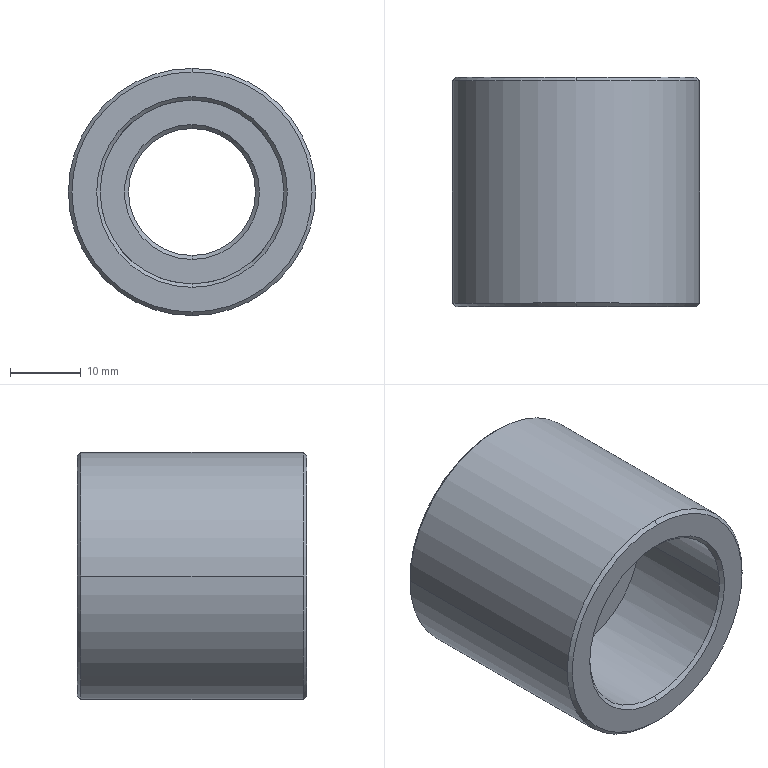Part | Creo | 1 solid | 17 faces | box 35 x 32.5 x 35 mm | volume 18391 mm3 | cone 8 | cylinder 6 | plane 3 | commonest cylinder face diameters 18 x2 26 x2 35 x2
STEP:
#1=CARTESIAN_POINT('',(203.5,-339.005,-225.));
#2=VERTEX_POINT('',#1);
#3=CARTESIAN_POINT('',(212.5,-339.005,-234.));
#4=VERTEX_POINT('',#3);
#5=CARTESIAN_POINT('',(212.5,-339.005,-225.));
#6=DIRECTION('',(0.,-1.,0.));
#7=DIRECTION('',(-1.,0.,0.));
#8=AXIS2_PLACEMENT_3D('',#5,#6,#7);
#9=CIRCLE('',#8,9.);
#10=EDGE_CURVE('',#2,#4,#9,.T.);
#11=ORIENTED_EDGE('',*,*,#10,.T.);
#12=CARTESIAN_POINT('',(221.5,-339.005,-225.));
#13=VERTEX_POINT('',#12);
#14=CARTESIAN_POINT('',(212.5,-339.005,-225.));
#15=DIRECTION('',(0.,-1.,0.));
#16=DIRECTION('',(0.,0.,-1.));
#17=AXIS2_PLACEMENT_3D('',#14,#15,#16);
#18=CIRCLE('',#17,9.);
#19=EDGE_CURVE('',#4,#13,#18,.T.);
#20=ORIENTED_EDGE('',*,*,#19,.T.);
#21=CARTESIAN_POINT('',(221.5,-354.455,-225.));
#22=VERTEX_POINT('',#21);
#23=CARTESIAN_POINT('',(221.5,-339.005,-225.));
#24=DIRECTION('',(0.,-1.,0.));
#25=VECTOR('',#24,15.45);
#26=LINE('',#23,#25);
#27=EDGE_CURVE('',#13,#22,#26,.T.);
#28=ORIENTED_EDGE('',*,*,#27,.T.);
#29=CARTESIAN_POINT('',(212.5,-354.455,-234.));
#30=VERTEX_POINT('',#29);
#31=CARTESIAN_POINT('',(212.5,-354.455,-225.));
#32=DIRECTION('',(0.,1.,0.));
#33=DIRECTION('',(1.,0.,0.));
#34=AXIS2_PLACEMENT_3D('',#31,#32,#33);
#35=CIRCLE('',#34,9.);
#36=EDGE_CURVE('',#22,#30,#35,.T.);
#37=ORIENTED_EDGE('',*,*,#36,.T.);
#38=CARTESIAN_POINT('',(203.5,-354.455,-225.));
#39=VERTEX_POINT('',#38);
#40=CARTESIAN_POINT('',(212.5,-354.455,-225.));
#41=DIRECTION('',(0.,1.,0.));
#42=DIRECTION('',(0.,0.,-1.));
#43=AXIS2_PLACEMENT_3D('',#40,#41,#42);
#44=CIRCLE('',#43,9.);
#45=EDGE_CURVE('',#30,#39,#44,.T.);
#46=ORIENTED_EDGE('',*,*,#45,.T.);
#47=CARTESIAN_POINT('',(203.5,-339.005,-225.));
#48=DIRECTION('',(0.,-1.,0.));
#49=VECTOR('',#48,15.45);
#50=LINE('',#47,#49);
#51=EDGE_CURVE('',#2,#39,#50,.T.);
#52=ORIENTED_EDGE('',*,*,#51,.F.);
#53=EDGE_LOOP('',(#11,#20,#28,#37,#46,#52));
#54=FACE_OUTER_BOUND('',#53,.F.);
#55=CARTESIAN_POINT('',(212.5,-374.005,-225.));
#56=DIRECTION('',(0.,-1.,0.));
#57=DIRECTION('',(-1.,0.,0.));
#58=AXIS2_PLACEMENT_3D('',#55,#56,#57);
#59=CYLINDRICAL_SURFACE('',#58,9.);
#60=ADVANCED_FACE('',(#54),#59,.F.);
#61=CARTESIAN_POINT('',(229.5,-339.005,-225.));
#62=VERTEX_POINT('',#61);
#63=CARTESIAN_POINT('',(212.5,-339.005,-242.));
#64=VERTEX_POINT('',#63);
#65=CARTESIAN_POINT('',(212.5,-339.005,-225.));
#66=DIRECTION('',(0.,1.,0.));
#67=DIRECTION('',(1.,0.,0.));
#68=AXIS2_PLACEMENT_3D('',#65,#66,#67);
#69=CIRCLE('',#68,17.);
#70=EDGE_CURVE('',#62,#64,#69,.T.);
#71=ORIENTED_EDGE('',*,*,#70,.F.);
#72=CARTESIAN_POINT('',(212.5,-339.005,-208.));
#73=VERTEX_POINT('',#72);
#74=CARTESIAN_POINT('',(212.5,-339.005,-225.));
#75=DIRECTION('',(0.,1.,0.));
#76=DIRECTION('',(0.,0.,1.));
#77=AXIS2_PLACEMENT_3D('',#74,#75,#76);
#78=CIRCLE('',#77,17.);
#79=EDGE_CURVE('',#73,#62,#78,.T.);
#80=ORIENTED_EDGE('',*,*,#79,.F.);
#81=CARTESIAN_POINT('',(195.5,-339.005,-225.));
#82=VERTEX_POINT('',#81);
#83=CARTESIAN_POINT('',(212.5,-339.005,-225.));
#84=DIRECTION('',(0.,1.,0.));
#85=DIRECTION('',(-1.,0.,0.));
#86=AXIS2_PLACEMENT_3D('',#83,#84,#85);
#87=CIRCLE('',#86,17.);
#88=EDGE_CURVE('',#82,#73,#87,.T.);
#89=ORIENTED_EDGE('',*,*,#88,.F.);
#90=CARTESIAN_POINT('',(212.5,-339.005,-225.));
#91=DIRECTION('',(0.,1.,0.));
#92=DIRECTION('',(0.,0.,-1.));
#93=AXIS2_PLACEMENT_3D('',#90,#91,#92);
#94=CIRCLE('',#93,17.);
#95=EDGE_CURVE('',#64,#82,#94,.T.);
#96=ORIENTED_EDGE('',*,*,#95,.F.);
#97=EDGE_LOOP('',(#71,#80,#89,#96));
#98=FACE_OUTER_BOUND('',#97,.F.);
#99=ORIENTED_EDGE('',*,*,#19,.F.);
#100=ORIENTED_EDGE('',*,*,#10,.F.);
#101=CARTESIAN_POINT('',(212.5,-339.005,-216.));
#102=VERTEX_POINT('',#101);
#103=CARTESIAN_POINT('',(212.5,-339.005,-225.));
#104=DIRECTION('',(0.,-1.,0.));
#105=DIRECTION('',(0.,0.,1.));
#106=AXIS2_PLACEMENT_3D('',#103,#104,#105);
#107=CIRCLE('',#106,9.);
#108=EDGE_CURVE('',#102,#2,#107,.T.);
#109=ORIENTED_EDGE('',*,*,#108,.F.);
#110=CARTESIAN_POINT('',(212.5,-339.005,-225.));
#111=DIRECTION('',(0.,-1.,0.));
#112=DIRECTION('',(1.,0.,0.));
#113=AXIS2_PLACEMENT_3D('',#110,#111,#112);
#114=CIRCLE('',#113,9.);
#115=EDGE_CURVE('',#13,#102,#114,.T.);
#116=ORIENTED_EDGE('',*,*,#115,.F.);
#117=EDGE_LOOP('',(#99,#100,#109,#116));
#118=FACE_BOUND('',#117,.F.);
#119=CARTESIAN_POINT('',(250.,-339.005,-375.));
#120=DIRECTION('',(0.,-1.,0.));
#121=DIRECTION('',(-1.,0.,0.));
#122=AXIS2_PLACEMENT_3D('',#119,#120,#121);
#123=PLANE('',#122);
#124=ADVANCED_FACE('',(#98,#118),#123,.F.);
#125=ORIENTED_EDGE('',*,*,#108,.T.);
#126=ORIENTED_EDGE('',*,*,#51,.T.);
#127=CARTESIAN_POINT('',(212.5,-354.455,-216.));
#128=VERTEX_POINT('',#127);
#129=CARTESIAN_POINT('',(212.5,-354.455,-225.));
#130=DIRECTION('',(0.,1.,0.));
#131=DIRECTION('',(-1.,0.,0.));
#132=AXIS2_PLACEMENT_3D('',#129,#130,#131);
#133=CIRCLE('',#132,9.);
#134=EDGE_CURVE('',#39,#128,#133,.T.);
#135=ORIENTED_EDGE('',*,*,#134,.T.);
#136=CARTESIAN_POINT('',(212.5,-354.455,-225.));
#137=DIRECTION('',(0.,1.,0.));
#138=DIRECTION('',(0.,0.,1.));
#139=AXIS2_PLACEMENT_3D('',#136,#137,#138);
#140=CIRCLE('',#139,9.);
#141=EDGE_CURVE('',#128,#22,#140,.T.);
#142=ORIENTED_EDGE('',*,*,#141,.T.);
#143=ORIENTED_EDGE('',*,*,#27,.F.);
#144=ORIENTED_EDGE('',*,*,#115,.T.);
#145=EDGE_LOOP('',(#125,#126,#135,#142,#143,#144));
#146=FACE_OUTER_BOUND('',#145,.F.);
#147=CARTESIAN_POINT('',(212.5,-374.005,-225.));
#148=DIRECTION('',(0.,-1.,0.));
#149=DIRECTION('',(-1.,0.,0.));
#150=AXIS2_PLACEMENT_3D('',#147,#148,#149);
#151=CYLINDRICAL_SURFACE('',#150,9.);
#152=ADVANCED_FACE('',(#146),#151,.F.);
#153=ORIENTED_EDGE('',*,*,#45,.F.);
#154=CARTESIAN_POINT('',(212.5,-355.005,-234.55));
#155=VERTEX_POINT('',#154);
#156=CARTESIAN_POINT('',(212.5,-354.455,-234.));
#157=DIRECTION('',(0.,-0.7071,-0.7071));
#158=VECTOR('',#157,0.7778);
#159=LINE('',#156,#158);
#160=EDGE_CURVE('',#30,#155,#159,.T.);
#161=ORIENTED_EDGE('',*,*,#160,.T.);
#162=CARTESIAN_POINT('',(212.5,-355.005,-215.45));
#163=VERTEX_POINT('',#162);
#164=CARTESIAN_POINT('',(212.5,-355.005,-225.));
#165=DIRECTION('',(0.,1.,0.));
#166=DIRECTION('',(0.,0.,-1.));
#167=AXIS2_PLACEMENT_3D('',#164,#165,#166);
#168=CIRCLE('',#167,9.55);
#169=EDGE_CURVE('',#155,#163,#168,.T.);
#170=ORIENTED_EDGE('',*,*,#169,.T.);
#171=CARTESIAN_POINT('',(212.5,-354.455,-216.));
#172=DIRECTION('',(0.,-0.7071,0.7071));
#173=VECTOR('',#172,0.7778);
#174=LINE('',#171,#173);
#175=EDGE_CURVE('',#128,#163,#174,.T.);
#176=ORIENTED_EDGE('',*,*,#175,.F.);
#177=ORIENTED_EDGE('',*,*,#134,.F.);
#178=EDGE_LOOP('',(#153,#161,#170,#176,#177));
#179=FACE_OUTER_BOUND('',#178,.F.);
#180=CARTESIAN_POINT('',(212.5,-354.73,-225.));
#181=DIRECTION('',(0.,-1.,0.));
#182=DIRECTION('',(0.,0.,1.));
#183=AXIS2_PLACEMENT_3D('',#180,#181,#182);
#184=CONICAL_SURFACE('',#183,9.275,45.);
#185=ADVANCED_FACE('',(#179),#184,.F.);
#186=ORIENTED_EDGE('',*,*,#141,.F.);
#187=ORIENTED_EDGE('',*,*,#175,.T.);
#188=CARTESIAN_POINT('',(222.05,-355.005,-225.));
#189=VERTEX_POINT('',#188);
#190=CARTESIAN_POINT('',(212.5,-355.005,-225.));
#191=DIRECTION('',(0.,1.,0.));
#192=DIRECTION('',(0.,0.,1.));
#193=AXIS2_PLACEMENT_3D('',#190,#191,#192);
#194=CIRCLE('',#193,9.55);
#195=EDGE_CURVE('',#163,#189,#194,.T.);
#196=ORIENTED_EDGE('',*,*,#195,.T.);
#197=CARTESIAN_POINT('',(212.5,-355.005,-225.));
#198=DIRECTION('',(0.,1.,0.));
#199=DIRECTION('',(1.,0.,0.));
#200=AXIS2_PLACEMENT_3D('',#197,#198,#199);
#201=CIRCLE('',#200,9.55);
#202=EDGE_CURVE('',#189,#155,#201,.T.);
#203=ORIENTED_EDGE('',*,*,#202,.T.);
#204=ORIENTED_EDGE('',*,*,#160,.F.);
#205=ORIENTED_EDGE('',*,*,#36,.F.);
#206=EDGE_LOOP('',(#186,#187,#196,#203,#204,#205));
#207=FACE_OUTER_BOUND('',#206,.F.);
#208=CARTESIAN_POINT('',(212.5,-354.73,-225.));
#209=DIRECTION('',(0.,-1.,0.));
#210=DIRECTION('',(0.,0.,1.));
#211=AXIS2_PLACEMENT_3D('',#208,#209,#210);
#212=CONICAL_SURFACE('',#211,9.275,45.);
#213=ADVANCED_FACE('',(#207),#212,.F.);
#214=CARTESIAN_POINT('',(199.5,-355.005,-225.));
#215=VERTEX_POINT('',#214);
#216=CARTESIAN_POINT('',(225.5,-355.005,-225.));
#217=VERTEX_POINT('',#216);
#218=CARTESIAN_POINT('',(212.5,-355.005,-225.));
#219=DIRECTION('',(0.,-1.,0.));
#220=DIRECTION('',(-1.,0.,0.));
#221=AXIS2_PLACEMENT_3D('',#218,#219,#220);
#222=CIRCLE('',#221,13.);
#223=EDGE_CURVE('',#215,#217,#222,.T.);
#224=ORIENTED_EDGE('',*,*,#223,.F.);
#225=CARTESIAN_POINT('',(212.5,-355.005,-225.));
#226=DIRECTION('',(0.,-1.,0.));
#227=DIRECTION('',(1.,0.,0.));
#228=AXIS2_PLACEMENT_3D('',#225,#226,#227);
#229=CIRCLE('',#228,13.);
#230=EDGE_CURVE('',#217,#215,#229,.T.);
#231=ORIENTED_EDGE('',*,*,#230,.F.);
#232=EDGE_LOOP('',(#224,#231));
#233=FACE_OUTER_BOUND('',#232,.F.);
#234=ORIENTED_EDGE('',*,*,#202,.F.);
#235=ORIENTED_EDGE('',*,*,#195,.F.);
#236=ORIENTED_EDGE('',*,*,#169,.F.);
#237=EDGE_LOOP('',(#234,#235,#236));
#238=FACE_BOUND('',#237,.F.);
#239=CARTESIAN_POINT('',(250.,-355.005,-375.));
#240=DIRECTION('',(0.,-1.,0.));
#241=DIRECTION('',(-1.,0.,0.));
#242=AXIS2_PLACEMENT_3D('',#239,#240,#241);
#243=PLANE('',#242);
#244=ADVANCED_FACE('',(#233,#238),#243,.T.);
#245=CARTESIAN_POINT('',(212.5,-371.005,-238.));
#246=VERTEX_POINT('',#245);
#247=CARTESIAN_POINT('',(199.5,-371.005,-225.));
#248=VERTEX_POINT('',#247);
#249=CARTESIAN_POINT('',(212.5,-371.005,-225.));
#250=DIRECTION('',(0.,1.,0.));
#251=DIRECTION('',(0.,0.,-1.));
#252=AXIS2_PLACEMENT_3D('',#249,#250,#251);
#253=CIRCLE('',#252,13.);
#254=EDGE_CURVE('',#246,#248,#253,.T.);
#255=ORIENTED_EDGE('',*,*,#254,.T.);
#256=CARTESIAN_POINT('',(199.5,-355.005,-225.));
#257=DIRECTION('',(0.,-1.,0.));
#258=VECTOR('',#257,16.);
#259=LINE('',#256,#258);
#260=EDGE_CURVE('',#215,#248,#259,.T.);
#261=ORIENTED_EDGE('',*,*,#260,.F.);
#262=ORIENTED_EDGE('',*,*,#223,.T.);
#263=CARTESIAN_POINT('',(225.5,-371.005,-225.));
#264=VERTEX_POINT('',#263);
#265=CARTESIAN_POINT('',(225.5,-355.005,-225.));
#266=DIRECTION('',(0.,-1.,0.));
#267=VECTOR('',#266,16.);
#268=LINE('',#265,#267);
#269=EDGE_CURVE('',#217,#264,#268,.T.);
#270=ORIENTED_EDGE('',*,*,#269,.T.);
#271=CARTESIAN_POINT('',(212.5,-371.005,-225.));
#272=DIRECTION('',(0.,1.,0.));
#273=DIRECTION('',(1.,0.,0.));
#274=AXIS2_PLACEMENT_3D('',#271,#272,#273);
#275=CIRCLE('',#274,13.);
#276=EDGE_CURVE('',#264,#246,#275,.T.);
#277=ORIENTED_EDGE('',*,*,#276,.T.);
#278=EDGE_LOOP('',(#255,#261,#262,#270,#277));
#279=FACE_OUTER_BOUND('',#278,.F.);
#280=CARTESIAN_POINT('',(212.5,-374.005,-225.));
#281=DIRECTION('',(0.,-1.,0.));
#282=DIRECTION('',(-1.,0.,0.));
#283=AXIS2_PLACEMENT_3D('',#280,#281,#282);
#284=CYLINDRICAL_SURFACE('',#283,13.);
#285=ADVANCED_FACE('',(#279),#284,.F.);
#286=CARTESIAN_POINT('',(212.5,-371.005,-212.));
#287=VERTEX_POINT('',#286);
#288=CARTESIAN_POINT('',(212.5,-371.005,-225.));
#289=DIRECTION('',(0.,1.,0.));
#290=DIRECTION('',(-1.,0.,0.));
#291=AXIS2_PLACEMENT_3D('',#288,#289,#290);
#292=CIRCLE('',#291,13.);
#293=EDGE_CURVE('',#248,#287,#292,.T.);
#294=ORIENTED_EDGE('',*,*,#293,.F.);
#295=ORIENTED_EDGE('',*,*,#254,.F.);
#296=CARTESIAN_POINT('',(212.5,-371.505,-238.5));
#297=VERTEX_POINT('',#296);
#298=CARTESIAN_POINT('',(212.5,-371.005,-238.));
#299=DIRECTION('',(0.,-0.7071,-0.7071));
#300=VECTOR('',#299,0.7071);
#301=LINE('',#298,#300);
#302=EDGE_CURVE('',#246,#297,#301,.T.);
#303=ORIENTED_EDGE('',*,*,#302,.T.);
#304=CARTESIAN_POINT('',(199.,-371.505,-225.));
#305=VERTEX_POINT('',#304);
#306=CARTESIAN_POINT('',(212.5,-371.505,-225.));
#307=DIRECTION('',(0.,1.,0.));
#308=DIRECTION('',(0.,0.,-1.));
#309=AXIS2_PLACEMENT_3D('',#306,#307,#308);
#310=CIRCLE('',#309,13.5);
#311=EDGE_CURVE('',#297,#305,#310,.T.);
#312=ORIENTED_EDGE('',*,*,#311,.T.);
#313=CARTESIAN_POINT('',(212.5,-371.505,-211.5));
#314=VERTEX_POINT('',#313);
#315=CARTESIAN_POINT('',(212.5,-371.505,-225.));
#316=DIRECTION('',(0.,1.,0.));
#317=DIRECTION('',(-1.,0.,-0.000000007));
#318=AXIS2_PLACEMENT_3D('',#315,#316,#317);
#319=CIRCLE('',#318,13.5);
#320=EDGE_CURVE('',#305,#314,#319,.T.);
#321=ORIENTED_EDGE('',*,*,#320,.T.);
#322=CARTESIAN_POINT('',(212.5,-371.005,-212.));
#323=DIRECTION('',(0.,-0.7071,0.7071));
#324=VECTOR('',#323,0.7071);
#325=LINE('',#322,#324);
#326=EDGE_CURVE('',#287,#314,#325,.T.);
#327=ORIENTED_EDGE('',*,*,#326,.F.);
#328=EDGE_LOOP('',(#294,#295,#303,#312,#321,#327));
#329=FACE_OUTER_BOUND('',#328,.F.);
#330=CARTESIAN_POINT('',(212.5,-371.255,-225.));
#331=DIRECTION('',(0.,-1.,0.));
#332=DIRECTION('',(0.,0.,1.));
#333=AXIS2_PLACEMENT_3D('',#330,#331,#332);
#334=CONICAL_SURFACE('',#333,13.25,45.);
#335=ADVANCED_FACE('',(#329),#334,.F.);
#336=CARTESIAN_POINT('',(212.5,-371.005,-225.));
#337=DIRECTION('',(0.,1.,0.));
#338=DIRECTION('',(0.,0.,1.));
#339=AXIS2_PLACEMENT_3D('',#336,#337,#338);
#340=CIRCLE('',#339,13.);
#341=EDGE_CURVE('',#287,#264,#340,.T.);
#342=ORIENTED_EDGE('',*,*,#341,.T.);
#343=ORIENTED_EDGE('',*,*,#269,.F.);
#344=ORIENTED_EDGE('',*,*,#230,.T.);
#345=ORIENTED_EDGE('',*,*,#260,.T.);
#346=ORIENTED_EDGE('',*,*,#293,.T.);
#347=EDGE_LOOP('',(#342,#343,#344,#345,#346));
#348=FACE_OUTER_BOUND('',#347,.F.);
#349=CARTESIAN_POINT('',(212.5,-374.005,-225.));
#350=DIRECTION('',(0.,-1.,0.));
#351=DIRECTION('',(-1.,0.,0.));
#352=AXIS2_PLACEMENT_3D('',#349,#350,#351);
#353=CYLINDRICAL_SURFACE('',#352,13.);
#354=ADVANCED_FACE('',(#348),#353,.F.);
#355=ORIENTED_EDGE('',*,*,#341,.F.);
#356=ORIENTED_EDGE('',*,*,#326,.T.);
#357=CARTESIAN_POINT('',(226.,-371.505,-225.));
#358=VERTEX_POINT('',#357);
#359=CARTESIAN_POINT('',(212.5,-371.505,-225.));
#360=DIRECTION('',(0.,1.,0.));
#361=DIRECTION('',(0.,0.,1.));
#362=AXIS2_PLACEMENT_3D('',#359,#360,#361);
#363=CIRCLE('',#362,13.5);
#364=EDGE_CURVE('',#314,#358,#363,.T.);
#365=ORIENTED_EDGE('',*,*,#364,.T.);
#366=CARTESIAN_POINT('',(212.5,-371.505,-225.));
#367=DIRECTION('',(0.,1.,0.));
#368=DIRECTION('',(1.,0.,0.000000007));
#369=AXIS2_PLACEMENT_3D('',#366,#367,#368);
#370=CIRCLE('',#369,13.5);
#371=EDGE_CURVE('',#358,#297,#370,.T.);
#372=ORIENTED_EDGE('',*,*,#371,.T.);
#373=ORIENTED_EDGE('',*,*,#302,.F.);
#374=ORIENTED_EDGE('',*,*,#276,.F.);
#375=EDGE_LOOP('',(#355,#356,#365,#372,#373,#374));
#376=FACE_OUTER_BOUND('',#375,.F.);
#377=CARTESIAN_POINT('',(212.5,-371.255,-225.));
#378=DIRECTION('',(0.,-1.,0.));
#379=DIRECTION('',(0.,0.,1.));
#380=AXIS2_PLACEMENT_3D('',#377,#378,#379);
#381=CONICAL_SURFACE('',#380,13.25,45.);
#382=ADVANCED_FACE('',(#376),#381,.F.);
#383=CARTESIAN_POINT('',(229.5,-371.505,-225.));
#384=VERTEX_POINT('',#383);
#385=CARTESIAN_POINT('',(212.5,-371.505,-208.));
#386=VERTEX_POINT('',#385);
#387=CARTESIAN_POINT('',(212.5,-371.505,-225.));
#388=DIRECTION('',(0.,-1.,0.));
#389=DIRECTION('',(1.,0.,-0.000000002));
#390=AXIS2_PLACEMENT_3D('',#387,#388,#389);
#391=CIRCLE('',#390,17.);
#392=EDGE_CURVE('',#384,#386,#391,.T.);
#393=ORIENTED_EDGE('',*,*,#392,.F.);
#394=CARTESIAN_POINT('',(212.5,-371.505,-242.));
#395=VERTEX_POINT('',#394);
#396=CARTESIAN_POINT('',(212.5,-371.505,-225.));
#397=DIRECTION('',(0.,-1.,0.));
#398=DIRECTION('',(0.,0.,-1.));
#399=AXIS2_PLACEMENT_3D('',#396,#397,#398);
#400=CIRCLE('',#399,17.);
#401=EDGE_CURVE('',#395,#384,#400,.T.);
#402=ORIENTED_EDGE('',*,*,#401,.F.);
#403=CARTESIAN_POINT('',(195.5,-371.505,-225.));
#404=VERTEX_POINT('',#403);
#405=CARTESIAN_POINT('',(212.5,-371.505,-225.));
#406=DIRECTION('',(0.,-1.,0.));
#407=DIRECTION('',(-1.,0.,0.000000002));
#408=AXIS2_PLACEMENT_3D('',#405,#406,#407);
#409=CIRCLE('',#408,17.);
#410=EDGE_CURVE('',#404,#395,#409,.T.);
#411=ORIENTED_EDGE('',*,*,#410,.F.);
#412=CARTESIAN_POINT('',(212.5,-371.505,-225.));
#413=DIRECTION('',(0.,-1.,0.));
#414=DIRECTION('',(0.,0.,1.));
#415=AXIS2_PLACEMENT_3D('',#412,#413,#414);
#416=CIRCLE('',#415,17.);
#417=EDGE_CURVE('',#386,#404,#416,.T.);
#418=ORIENTED_EDGE('',*,*,#417,.F.);
#419=EDGE_LOOP('',(#393,#402,#411,#418));
#420=FACE_OUTER_BOUND('',#419,.F.);
#421=ORIENTED_EDGE('',*,*,#320,.F.);
#422=ORIENTED_EDGE('',*,*,#311,.F.);
#423=ORIENTED_EDGE('',*,*,#371,.F.);
#424=ORIENTED_EDGE('',*,*,#364,.F.);
#425=EDGE_LOOP('',(#421,#422,#423,#424));
#426=FACE_BOUND('',#425,.F.);
#427=CARTESIAN_POINT('',(250.,-371.505,-375.));
#428=DIRECTION('',(0.,-1.,0.));
#429=DIRECTION('',(-1.,0.,0.));
#430=AXIS2_PLACEMENT_3D('',#427,#428,#429);
#431=PLANE('',#430);
#432=ADVANCED_FACE('',(#420,#426),#431,.T.);
#433=ORIENTED_EDGE('',*,*,#401,.T.);
#434=ORIENTED_EDGE('',*,*,#392,.T.);
#435=CARTESIAN_POINT('',(212.5,-371.005,-207.5));
#436=VERTEX_POINT('',#435);
#437=CARTESIAN_POINT('',(212.5,-371.505,-208.));
#438=DIRECTION('',(0.,0.7071,0.7071));
#439=VECTOR('',#438,0.7071);
#440=LINE('',#437,#439);
#441=EDGE_CURVE('',#386,#436,#440,.T.);
#442=ORIENTED_EDGE('',*,*,#441,.T.);
#443=CARTESIAN_POINT('',(230.,-371.005,-225.));
#444=VERTEX_POINT('',#443);
#445=CARTESIAN_POINT('',(212.5,-371.005,-225.));
#446=DIRECTION('',(0.,-1.,0.));
#447=DIRECTION('',(1.,0.,0.));
#448=AXIS2_PLACEMENT_3D('',#445,#446,#447);
#449=CIRCLE('',#448,17.5);
#450=EDGE_CURVE('',#444,#436,#449,.T.);
#451=ORIENTED_EDGE('',*,*,#450,.F.);
#452=CARTESIAN_POINT('',(212.5,-371.005,-242.5));
#453=VERTEX_POINT('',#452);
#454=CARTESIAN_POINT('',(212.5,-371.005,-225.));
#455=DIRECTION('',(0.,-1.,0.));
#456=DIRECTION('',(0.,0.,-1.));
#457=AXIS2_PLACEMENT_3D('',#454,#455,#456);
#458=CIRCLE('',#457,17.5);
#459=EDGE_CURVE('',#453,#444,#458,.T.);
#460=ORIENTED_EDGE('',*,*,#459,.F.);
#461=CARTESIAN_POINT('',(212.5,-371.505,-242.));
#462=DIRECTION('',(0.,0.7071,-0.7071));
#463=VECTOR('',#462,0.7071);
#464=LINE('',#461,#463);
#465=EDGE_CURVE('',#395,#453,#464,.T.);
#466=ORIENTED_EDGE('',*,*,#465,.F.);
#467=EDGE_LOOP('',(#433,#434,#442,#451,#460,#466));
#468=FACE_OUTER_BOUND('',#467,.F.);
#469=CARTESIAN_POINT('',(212.5,-371.255,-225.));
#470=DIRECTION('',(0.,1.,0.));
#471=DIRECTION('',(0.,0.,1.));
#472=AXIS2_PLACEMENT_3D('',#469,#470,#471);
#473=CONICAL_SURFACE('',#472,17.25,45.);
#474=ADVANCED_FACE('',(#468),#473,.T.);
#475=ORIENTED_EDGE('',*,*,#410,.T.);
#476=ORIENTED_EDGE('',*,*,#465,.T.);
#477=CARTESIAN_POINT('',(195.,-371.005,-225.));
#478=VERTEX_POINT('',#477);
#479=CARTESIAN_POINT('',(212.5,-371.005,-225.));
#480=DIRECTION('',(0.,-1.,0.));
#481=DIRECTION('',(-1.,0.,0.));
#482=AXIS2_PLACEMENT_3D('',#479,#480,#481);
#483=CIRCLE('',#482,17.5);
#484=EDGE_CURVE('',#478,#453,#483,.T.);
#485=ORIENTED_EDGE('',*,*,#484,.F.);
#486=CARTESIAN_POINT('',(212.5,-371.005,-225.));
#487=DIRECTION('',(0.,-1.,0.));
#488=DIRECTION('',(0.,0.,1.));
#489=AXIS2_PLACEMENT_3D('',#486,#487,#488);
#490=CIRCLE('',#489,17.5);
#491=EDGE_CURVE('',#436,#478,#490,.T.);
#492=ORIENTED_EDGE('',*,*,#491,.F.);
#493=ORIENTED_EDGE('',*,*,#441,.F.);
#494=ORIENTED_EDGE('',*,*,#417,.T.);
#495=EDGE_LOOP('',(#475,#476,#485,#492,#493,#494));
#496=FACE_OUTER_BOUND('',#495,.F.);
#497=CARTESIAN_POINT('',(212.5,-371.255,-225.));
#498=DIRECTION('',(0.,1.,0.));
#499=DIRECTION('',(0.,0.,1.));
#500=AXIS2_PLACEMENT_3D('',#497,#498,#499);
#501=CONICAL_SURFACE('',#500,17.25,45.);
#502=ADVANCED_FACE('',(#496),#501,.T.);
#503=CARTESIAN_POINT('',(212.5,-339.505,-242.5));
#504=VERTEX_POINT('',#503);
#505=CARTESIAN_POINT('',(195.,-339.505,-225.));
#506=VERTEX_POINT('',#505);
#507=CARTESIAN_POINT('',(212.5,-339.505,-225.));
#508=DIRECTION('',(0.,1.,0.));
#509=DIRECTION('',(-0.000000003,0.,-1.));
#510=AXIS2_PLACEMENT_3D('',#507,#508,#509);
#511=CIRCLE('',#510,17.5);
#512=EDGE_CURVE('',#504,#506,#511,.T.);
#513=ORIENTED_EDGE('',*,*,#512,.T.);
#514=CARTESIAN_POINT('',(195.,-339.505,-225.));
#515=DIRECTION('',(0.000000011,-1.,0.));
#516=VECTOR('',#515,31.5);
#517=LINE('',#514,#516);
#518=EDGE_CURVE('',#506,#478,#517,.T.);
#519=ORIENTED_EDGE('',*,*,#518,.T.);
#520=ORIENTED_EDGE('',*,*,#484,.T.);
#521=ORIENTED_EDGE('',*,*,#459,.T.);
#522=CARTESIAN_POINT('',(230.,-339.505,-225.));
#523=VERTEX_POINT('',#522);
#524=CARTESIAN_POINT('',(230.,-339.505,-225.));
#525=DIRECTION('',(-0.000000011,-1.,0.000000001));
#526=VECTOR('',#525,31.5);
#527=LINE('',#524,#526);
#528=EDGE_CURVE('',#523,#444,#527,.T.);
#529=ORIENTED_EDGE('',*,*,#528,.F.);
#530=CARTESIAN_POINT('',(212.5,-339.505,-225.));
#531=DIRECTION('',(0.,1.,0.));
#532=DIRECTION('',(1.,0.,0.));
#533=AXIS2_PLACEMENT_3D('',#530,#531,#532);
#534=CIRCLE('',#533,17.5);
#535=EDGE_CURVE('',#523,#504,#534,.T.);
#536=ORIENTED_EDGE('',*,*,#535,.T.);
#537=EDGE_LOOP('',(#513,#519,#520,#521,#529,#536));
#538=FACE_OUTER_BOUND('',#537,.F.);
#539=CARTESIAN_POINT('',(212.5,-339.005,-225.));
#540=DIRECTION('',(0.,-1.,0.));
#541=DIRECTION('',(-1.,0.,0.));
#542=AXIS2_PLACEMENT_3D('',#539,#540,#541);
#543=CYLINDRICAL_SURFACE('',#542,17.5);
#544=ADVANCED_FACE('',(#538),#543,.T.);
#545=ORIENTED_EDGE('',*,*,#88,.T.);
#546=CARTESIAN_POINT('',(212.5,-339.505,-207.5));
#547=VERTEX_POINT('',#546);
#548=CARTESIAN_POINT('',(212.5,-339.005,-208.));
#549=DIRECTION('',(0.000000024,-0.7071,0.7071));
#550=VECTOR('',#549,0.7071);
#551=LINE('',#548,#550);
#552=EDGE_CURVE('',#73,#547,#551,.T.);
#553=ORIENTED_EDGE('',*,*,#552,.T.);
#554=CARTESIAN_POINT('',(212.5,-339.505,-225.));
#555=DIRECTION('',(0.,1.,0.));
#556=DIRECTION('',(-1.,0.,0.));
#557=AXIS2_PLACEMENT_3D('',#554,#555,#556);
#558=CIRCLE('',#557,17.5);
#559=EDGE_CURVE('',#506,#547,#558,.T.);
#560=ORIENTED_EDGE('',*,*,#559,.F.);
#561=ORIENTED_EDGE('',*,*,#512,.F.);
#562=CARTESIAN_POINT('',(212.5,-339.005,-242.));
#563=DIRECTION('',(-0.000000024,-0.7071,-0.7071));
#564=VECTOR('',#563,0.7071);
#565=LINE('',#562,#564);
#566=EDGE_CURVE('',#64,#504,#565,.T.);
#567=ORIENTED_EDGE('',*,*,#566,.F.);
#568=ORIENTED_EDGE('',*,*,#95,.T.);
#569=EDGE_LOOP('',(#545,#553,#560,#561,#567,#568));
#570=FACE_OUTER_BOUND('',#569,.F.);
#571=CARTESIAN_POINT('',(212.5,-339.255,-225.));
#572=DIRECTION('',(0.,-1.,0.));
#573=DIRECTION('',(0.,0.,1.));
#574=AXIS2_PLACEMENT_3D('',#571,#572,#573);
#575=CONICAL_SURFACE('',#574,17.25,45.);
#576=ADVANCED_FACE('',(#570),#575,.T.);
#577=ORIENTED_EDGE('',*,*,#79,.T.);
#578=ORIENTED_EDGE('',*,*,#70,.T.);
#579=ORIENTED_EDGE('',*,*,#566,.T.);
#580=ORIENTED_EDGE('',*,*,#535,.F.);
#581=CARTESIAN_POINT('',(212.5,-339.505,-225.));
#582=DIRECTION('',(0.,1.,0.));
#583=DIRECTION('',(0.000000003,0.,1.));
#584=AXIS2_PLACEMENT_3D('',#581,#582,#583);
#585=CIRCLE('',#584,17.5);
#586=EDGE_CURVE('',#547,#523,#585,.T.);
#587=ORIENTED_EDGE('',*,*,#586,.F.);
#588=ORIENTED_EDGE('',*,*,#552,.F.);
#589=EDGE_LOOP('',(#577,#578,#579,#580,#587,#588));
#590=FACE_OUTER_BOUND('',#589,.F.);
#591=CARTESIAN_POINT('',(212.5,-339.255,-225.));
#592=DIRECTION('',(0.,-1.,0.));
#593=DIRECTION('',(0.,0.,1.));
#594=AXIS2_PLACEMENT_3D('',#591,#592,#593);
#595=CONICAL_SURFACE('',#594,17.25,45.);
#596=ADVANCED_FACE('',(#590),#595,.T.);
#597=ORIENTED_EDGE('',*,*,#586,.T.);
#598=ORIENTED_EDGE('',*,*,#528,.T.);
#599=ORIENTED_EDGE('',*,*,#450,.T.);
#600=ORIENTED_EDGE('',*,*,#491,.T.);
#601=ORIENTED_EDGE('',*,*,#518,.F.);
#602=ORIENTED_EDGE('',*,*,#559,.T.);
#603=EDGE_LOOP('',(#597,#598,#599,#600,#601,#602));
#604=FACE_OUTER_BOUND('',#603,.F.);
#605=CARTESIAN_POINT('',(212.5,-339.005,-225.));
#606=DIRECTION('',(0.,-1.,0.));
#607=DIRECTION('',(-1.,0.,0.));
#608=AXIS2_PLACEMENT_3D('',#605,#606,#607);
#609=CYLINDRICAL_SURFACE('',#608,17.5);
#610=ADVANCED_FACE('',(#604),#609,.T.);
#611=CLOSED_SHELL('',(#60,#124,#152,#185,#213,#244,#285,#335,#354,#382,#432,#474,#502,#544,#576,#596,#610));
#612=MANIFOLD_SOLID_BREP('',#611);
#613=(LENGTH_UNIT()NAMED_UNIT(*)SI_UNIT(.MILLI.,.METRE.));
#614=UNCERTAINTY_MEASURE_WITH_UNIT(LENGTH_MEASURE(0.005921),#613,'','');
#615=(NAMED_UNIT(*)PLANE_ANGLE_UNIT()SI_UNIT($,.RADIAN.));
#616=PLANE_ANGLE_MEASURE_WITH_UNIT(PLANE_ANGLE_MEASURE(0.01745),#615);
#617=(CONVERSION_BASED_UNIT('DEGREE',#616)NAMED_UNIT(*)PLANE_ANGLE_UNIT());
#618=(NAMED_UNIT(*)SI_UNIT($,.STERADIAN.)SOLID_ANGLE_UNIT());
#619=(GEOMETRIC_REPRESENTATION_CONTEXT(3)GLOBAL_UNCERTAINTY_ASSIGNED_CONTEXT((#614))GLOBAL_UNIT_ASSIGNED_CONTEXT((#613,#617,#618))REPRESENTATION_CONTEXT('',''));
#620=ADVANCED_BREP_SHAPE_REPRESENTATION('',(#612),#619);